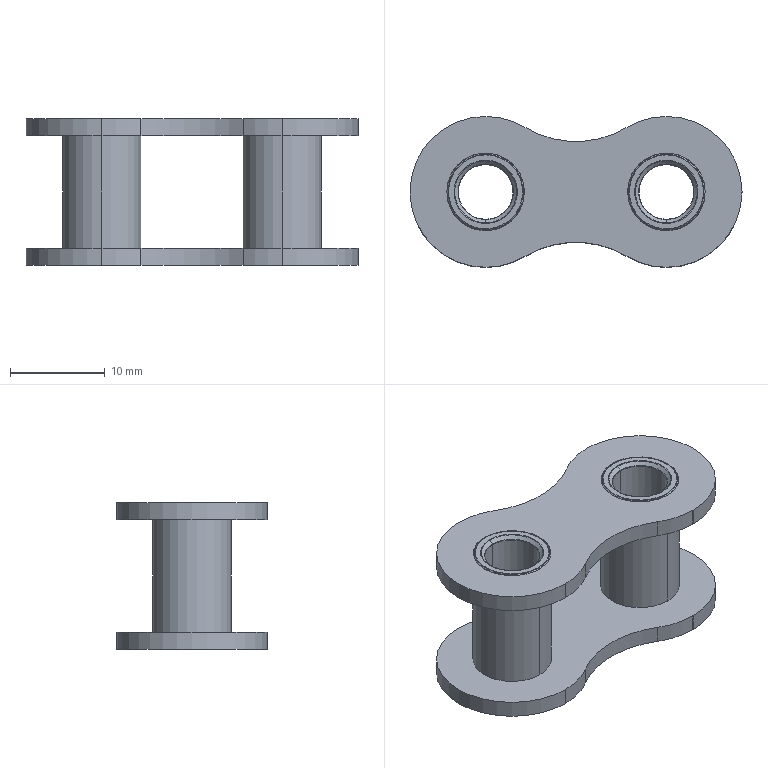Part | STEP file | 12b-1_02 | 1 solid | 88 faces | box 35 x 15.9 x 15.6 mm | volume 2080 mm3 | cylinder 32 | torus 20 | cone 16 | plane 16 | spline 4 | commonest cylinder face diameters 15.9 x12 8.18 x8 5.8 x4 8.29 x4 20.8 x4